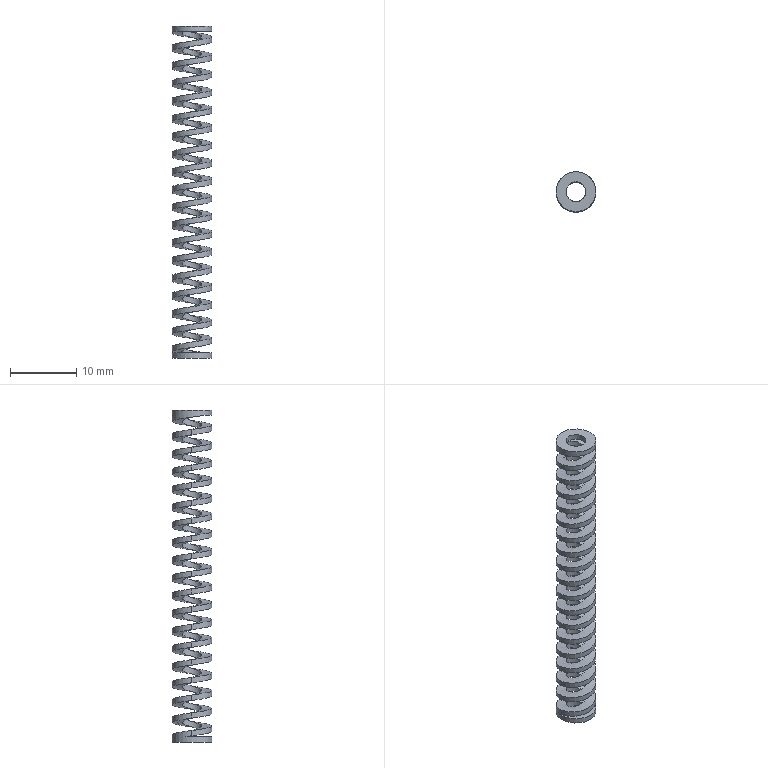Part | STEP file | 1 solid | 44 faces | box 6 x 6 x 50 mm | volume 346.471 mm3 | cylinder 38 | plane 4 | spline 2 | commonest cylinder face diameters 3 x19 6 x19